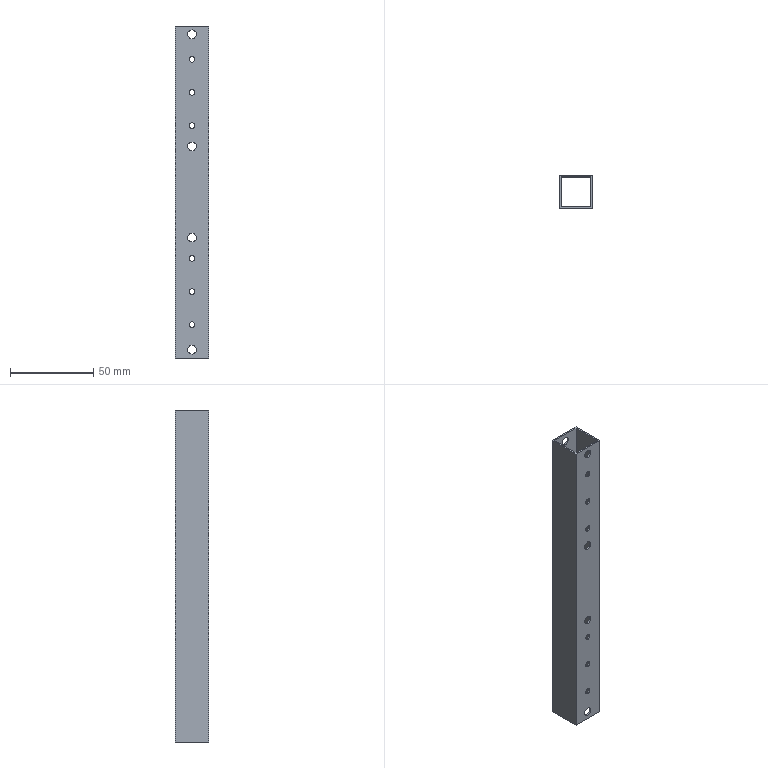Part | SolidWorks | features BaseBody 1 | 1 solid | 50 faces | box 20 x 20 x 200 mm | volume 14915 mm3 | cylinder 40 | plane 10 | commonest cylinder face diameters 3.5 x24 5.2 x16